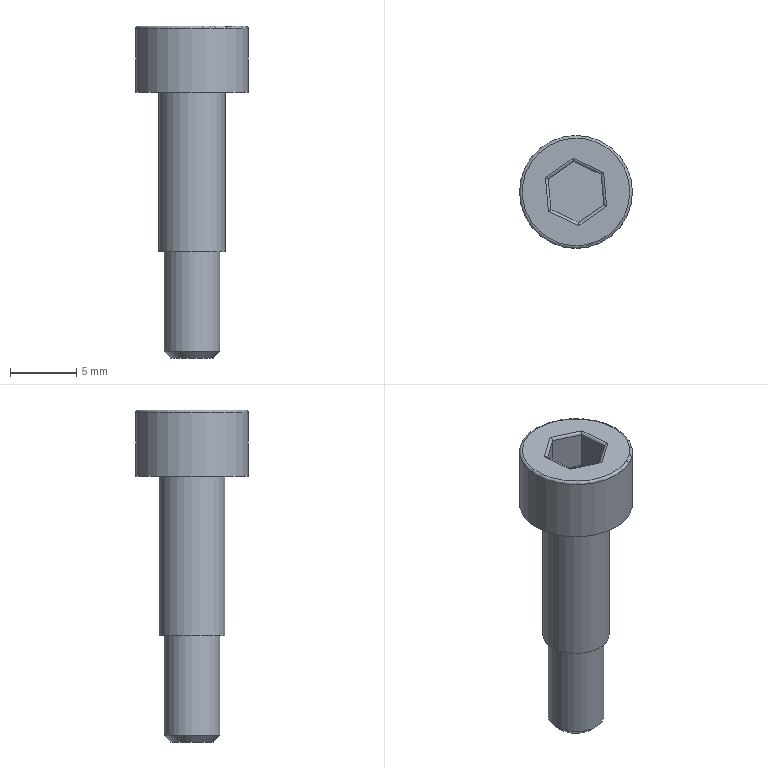Part | STEP file | 200 mesh_id970_x | 1 solid | 22 faces | box 8.5 x 8.5 x 25 mm | volume 586.744 mm3 | plane 11 | cylinder 9 | torus 1 | cone 1 | commonest cylinder face diameters 0.4 x6 4.2 x1 5 x1 8.5 x1
STEP:
#1=CARTESIAN_POINT('',(-16735.184,-4091.769,73.43));
#2=VERTEX_POINT('',#1);
#3=CARTESIAN_POINT('',(-16732.684,-4091.769,73.43));
#4=DIRECTION('',(0.,0.,1.));
#5=DIRECTION('',(-1.,0.,0.));
#6=AXIS2_PLACEMENT_3D('',#3,#4,#5);
#7=CIRCLE('',#6,2.5);
#8=EDGE_CURVE('',#2,#2,#7,.T.);
#9=ORIENTED_EDGE('',*,*,#8,.T.);
#10=EDGE_LOOP('',(#9));
#11=FACE_BOUND('',#10,.T.);
#12=CARTESIAN_POINT('',(-16728.434,-4091.769,73.43));
#13=VERTEX_POINT('',#12);
#14=CARTESIAN_POINT('',(-16732.684,-4091.769,73.43));
#15=DIRECTION('',(0.,0.,1.));
#16=DIRECTION('',(1.,0.,0.));
#17=AXIS2_PLACEMENT_3D('',#14,#15,#16);
#18=CIRCLE('',#17,4.25);
#19=EDGE_CURVE('',#13,#13,#18,.T.);
#20=ORIENTED_EDGE('',*,*,#19,.F.);
#21=EDGE_LOOP('',(#20));
#22=FACE_BOUND('',#21,.T.);
#23=CARTESIAN_POINT('',(-16732.684,-4091.769,73.43));
#24=DIRECTION('',(0.,0.,-1.));
#25=DIRECTION('',(-1.,0.,0.));
#26=AXIS2_PLACEMENT_3D('',#23,#24,#25);
#27=PLANE('',#26);
#28=ADVANCED_FACE('',(#11,#22),#27,.T.);
#29=CARTESIAN_POINT('',(-16734.986,-4090.696,78.43));
#30=VERTEX_POINT('',#29);
#31=CARTESIAN_POINT('',(-16732.905,-4089.239,78.43));
#32=VERTEX_POINT('',#31);
#33=CARTESIAN_POINT('',(-16733.946,-4089.967,78.43));
#34=DIRECTION('',(0.8192,0.5736,0.));
#35=VECTOR('',#34,1.);
#36=LINE('',#33,#35);
#37=EDGE_CURVE('',#30,#32,#36,.T.);
#38=ORIENTED_EDGE('',*,*,#37,.T.);
#39=CARTESIAN_POINT('',(-16730.603,-4090.312,78.43));
#40=VERTEX_POINT('',#39);
#41=CARTESIAN_POINT('',(-16731.754,-4089.775,78.43));
#42=DIRECTION('',(0.9063,-0.4226,0.));
#43=VECTOR('',#42,1.);
#44=LINE('',#41,#43);
#45=EDGE_CURVE('',#32,#40,#44,.T.);
#46=ORIENTED_EDGE('',*,*,#45,.T.);
#47=CARTESIAN_POINT('',(-16730.382,-4092.843,78.43));
#48=VERTEX_POINT('',#47);
#49=CARTESIAN_POINT('',(-16730.492,-4091.577,78.43));
#50=DIRECTION('',(0.08716,-0.9962,0.));
#51=VECTOR('',#50,1.);
#52=LINE('',#49,#51);
#53=EDGE_CURVE('',#40,#48,#52,.T.);
#54=ORIENTED_EDGE('',*,*,#53,.T.);
#55=CARTESIAN_POINT('',(-16732.463,-4094.3,78.43));
#56=VERTEX_POINT('',#55);
#57=CARTESIAN_POINT('',(-16731.422,-4093.571,78.43));
#58=DIRECTION('',(-0.8192,-0.5736,0.));
#59=VECTOR('',#58,1.);
#60=LINE('',#57,#59);
#61=EDGE_CURVE('',#48,#56,#60,.T.);
#62=ORIENTED_EDGE('',*,*,#61,.T.);
#63=CARTESIAN_POINT('',(-16734.765,-4093.226,78.43));
#64=VERTEX_POINT('',#63);
#65=CARTESIAN_POINT('',(-16733.614,-4093.763,78.43));
#66=DIRECTION('',(-0.9063,0.4226,0.));
#67=VECTOR('',#66,1.);
#68=LINE('',#65,#67);
#69=EDGE_CURVE('',#56,#64,#68,.T.);
#70=ORIENTED_EDGE('',*,*,#69,.T.);
#71=CARTESIAN_POINT('',(-16734.876,-4091.961,78.43));
#72=DIRECTION('',(-0.08716,0.9962,0.));
#73=VECTOR('',#72,1.);
#74=LINE('',#71,#73);
#75=EDGE_CURVE('',#64,#30,#74,.T.);
#76=ORIENTED_EDGE('',*,*,#75,.T.);
#77=EDGE_LOOP('',(#38,#46,#54,#62,#70,#76));
#78=FACE_BOUND('',#77,.T.);
#79=CARTESIAN_POINT('',(-16728.634,-4091.769,78.43));
#80=VERTEX_POINT('',#79);
#81=CARTESIAN_POINT('',(-16732.684,-4091.769,78.43));
#82=DIRECTION('',(0.,0.,1.));
#83=DIRECTION('',(1.,0.,0.));
#84=AXIS2_PLACEMENT_3D('',#81,#82,#83);
#85=CIRCLE('',#84,4.05);
#86=EDGE_CURVE('',#80,#80,#85,.T.);
#87=ORIENTED_EDGE('',*,*,#86,.T.);
#88=EDGE_LOOP('',(#87));
#89=FACE_BOUND('',#88,.T.);
#90=CARTESIAN_POINT('',(-16732.684,-4091.769,78.43));
#91=DIRECTION('',(0.,0.,1.));
#92=DIRECTION('',(1.,0.,0.));
#93=AXIS2_PLACEMENT_3D('',#90,#91,#92);
#94=PLANE('',#93);
#95=ADVANCED_FACE('',(#78,#89),#94,.T.);
#96=CARTESIAN_POINT('',(-16728.434,-4091.769,78.23));
#97=VERTEX_POINT('',#96);
#98=CARTESIAN_POINT('',(-16732.684,-4091.769,78.23));
#99=DIRECTION('',(0.,0.,-1.));
#100=DIRECTION('',(1.,0.,0.));
#101=AXIS2_PLACEMENT_3D('',#98,#99,#100);
#102=CIRCLE('',#101,4.25);
#103=EDGE_CURVE('',#97,#97,#102,.T.);
#104=ORIENTED_EDGE('',*,*,#103,.T.);
#105=EDGE_LOOP('',(#104));
#106=FACE_BOUND('',#105,.T.);
#107=ORIENTED_EDGE('',*,*,#19,.T.);
#108=EDGE_LOOP('',(#107));
#109=FACE_BOUND('',#108,.T.);
#110=CARTESIAN_POINT('',(-16732.684,-4091.769,73.43));
#111=DIRECTION('',(0.,0.,1.));
#112=DIRECTION('',(1.,0.,0.));
#113=AXIS2_PLACEMENT_3D('',#110,#111,#112);
#114=CYLINDRICAL_SURFACE('',#113,4.25);
#115=ADVANCED_FACE('',(#106,#109),#114,.T.);
#116=ORIENTED_EDGE('',*,*,#86,.F.);
#117=EDGE_LOOP('',(#116));
#118=FACE_BOUND('',#117,.T.);
#119=ORIENTED_EDGE('',*,*,#103,.F.);
#120=EDGE_LOOP('',(#119));
#121=FACE_BOUND('',#120,.T.);
#122=CARTESIAN_POINT('',(-16732.684,-4091.769,78.23));
#123=DIRECTION('',(0.,0.,1.));
#124=DIRECTION('',(1.,0.,0.));
#125=AXIS2_PLACEMENT_3D('',#122,#123,#124);
#126=TOROIDAL_SURFACE('',#125,4.05,0.2);
#127=ADVANCED_FACE('',(#118,#121),#126,.T.);
#128=CARTESIAN_POINT('',(-16730.591,-4092.745,78.23));
#129=VERTEX_POINT('',#128);
#130=CARTESIAN_POINT('',(-16730.591,-4092.745,75.43));
#131=VERTEX_POINT('',#130);
#132=CARTESIAN_POINT('',(-16730.591,-4092.745,75.43));
#133=DIRECTION('',(0.,0.,-1.));
#134=VECTOR('',#133,1.);
#135=LINE('',#132,#134);
#136=EDGE_CURVE('',#129,#131,#135,.T.);
#137=ORIENTED_EDGE('',*,*,#136,.F.);
#138=CARTESIAN_POINT('',(-16730.792,-4090.445,78.23));
#139=VERTEX_POINT('',#138);
#140=CARTESIAN_POINT('',(-16730.792,-4090.445,78.23));
#141=DIRECTION('',(-0.08716,0.9962,0.));
#142=VECTOR('',#141,1.);
#143=LINE('',#140,#142);
#144=EDGE_CURVE('',#129,#139,#143,.T.);
#145=ORIENTED_EDGE('',*,*,#144,.T.);
#146=CARTESIAN_POINT('',(-16730.792,-4090.445,75.43));
#147=VERTEX_POINT('',#146);
#148=CARTESIAN_POINT('',(-16730.792,-4090.445,75.43));
#149=DIRECTION('',(0.,0.,-1.));
#150=VECTOR('',#149,1.);
#151=LINE('',#148,#150);
#152=EDGE_CURVE('',#139,#147,#151,.T.);
#153=ORIENTED_EDGE('',*,*,#152,.T.);
#154=CARTESIAN_POINT('',(-16730.792,-4090.445,75.43));
#155=DIRECTION('',(-0.08716,0.9962,0.));
#156=VECTOR('',#155,1.);
#157=LINE('',#154,#156);
#158=EDGE_CURVE('',#131,#147,#157,.T.);
#159=ORIENTED_EDGE('',*,*,#158,.F.);
#160=EDGE_LOOP('',(#137,#145,#153,#159));
#161=FACE_OUTER_BOUND('',#160,.T.);
#162=CARTESIAN_POINT('',(-16730.792,-4090.445,75.43));
#163=DIRECTION('',(-0.9962,-0.08716,0.));
#164=DIRECTION('',(0.08716,-0.9962,0.));
#165=AXIS2_PLACEMENT_3D('',#162,#163,#164);
#166=PLANE('',#165);
#167=ADVANCED_FACE('',(#161),#166,.T.);
#168=CARTESIAN_POINT('',(-16732.483,-4094.07,78.23));
#169=VERTEX_POINT('',#168);
#170=CARTESIAN_POINT('',(-16732.483,-4094.07,75.43));
#171=VERTEX_POINT('',#170);
#172=CARTESIAN_POINT('',(-16732.483,-4094.07,75.43));
#173=DIRECTION('',(0.,0.,-1.));
#174=VECTOR('',#173,1.);
#175=LINE('',#172,#174);
#176=EDGE_CURVE('',#169,#171,#175,.T.);
#177=ORIENTED_EDGE('',*,*,#176,.F.);
#178=CARTESIAN_POINT('',(-16730.591,-4092.745,78.23));
#179=DIRECTION('',(0.8192,0.5736,0.));
#180=VECTOR('',#179,1.);
#181=LINE('',#178,#180);
#182=EDGE_CURVE('',#169,#129,#181,.T.);
#183=ORIENTED_EDGE('',*,*,#182,.T.);
#184=ORIENTED_EDGE('',*,*,#136,.T.);
#185=CARTESIAN_POINT('',(-16730.591,-4092.745,75.43));
#186=DIRECTION('',(0.8192,0.5736,0.));
#187=VECTOR('',#186,1.);
#188=LINE('',#185,#187);
#189=EDGE_CURVE('',#171,#131,#188,.T.);
#190=ORIENTED_EDGE('',*,*,#189,.F.);
#191=EDGE_LOOP('',(#177,#183,#184,#190));
#192=FACE_OUTER_BOUND('',#191,.T.);
#193=CARTESIAN_POINT('',(-16730.591,-4092.745,75.43));
#194=DIRECTION('',(-0.5736,0.8192,0.));
#195=DIRECTION('',(-0.8192,-0.5736,0.));
#196=AXIS2_PLACEMENT_3D('',#193,#194,#195);
#197=PLANE('',#196);
#198=ADVANCED_FACE('',(#192),#197,.T.);
#199=CARTESIAN_POINT('',(-16734.576,-4093.094,78.23));
#200=VERTEX_POINT('',#199);
#201=CARTESIAN_POINT('',(-16734.576,-4093.094,75.43));
#202=VERTEX_POINT('',#201);
#203=CARTESIAN_POINT('',(-16734.576,-4093.094,75.43));
#204=DIRECTION('',(0.,0.,-1.));
#205=VECTOR('',#204,1.);
#206=LINE('',#203,#205);
#207=EDGE_CURVE('',#200,#202,#206,.T.);
#208=ORIENTED_EDGE('',*,*,#207,.F.);
#209=CARTESIAN_POINT('',(-16732.483,-4094.07,78.23));
#210=DIRECTION('',(0.9063,-0.4226,0.));
#211=VECTOR('',#210,1.);
#212=LINE('',#209,#211);
#213=EDGE_CURVE('',#200,#169,#212,.T.);
#214=ORIENTED_EDGE('',*,*,#213,.T.);
#215=ORIENTED_EDGE('',*,*,#176,.T.);
#216=CARTESIAN_POINT('',(-16732.483,-4094.07,75.43));
#217=DIRECTION('',(0.9063,-0.4226,0.));
#218=VECTOR('',#217,1.);
#219=LINE('',#216,#218);
#220=EDGE_CURVE('',#202,#171,#219,.T.);
#221=ORIENTED_EDGE('',*,*,#220,.F.);
#222=EDGE_LOOP('',(#208,#214,#215,#221));
#223=FACE_OUTER_BOUND('',#222,.T.);
#224=CARTESIAN_POINT('',(-16732.483,-4094.07,75.43));
#225=DIRECTION('',(0.4226,0.9063,0.));
#226=DIRECTION('',(-0.9063,0.4226,0.));
#227=AXIS2_PLACEMENT_3D('',#224,#225,#226);
#228=PLANE('',#227);
#229=ADVANCED_FACE('',(#223),#228,.T.);
#230=CARTESIAN_POINT('',(-16734.777,-4090.793,78.23));
#231=VERTEX_POINT('',#230);
#232=CARTESIAN_POINT('',(-16734.777,-4090.793,75.43));
#233=VERTEX_POINT('',#232);
#234=CARTESIAN_POINT('',(-16734.777,-4090.793,75.43));
#235=DIRECTION('',(0.,0.,-1.));
#236=VECTOR('',#235,1.);
#237=LINE('',#234,#236);
#238=EDGE_CURVE('',#231,#233,#237,.T.);
#239=ORIENTED_EDGE('',*,*,#238,.F.);
#240=CARTESIAN_POINT('',(-16734.576,-4093.094,78.23));
#241=DIRECTION('',(0.08716,-0.9962,0.));
#242=VECTOR('',#241,1.);
#243=LINE('',#240,#242);
#244=EDGE_CURVE('',#231,#200,#243,.T.);
#245=ORIENTED_EDGE('',*,*,#244,.T.);
#246=ORIENTED_EDGE('',*,*,#207,.T.);
#247=CARTESIAN_POINT('',(-16734.576,-4093.094,75.43));
#248=DIRECTION('',(0.08716,-0.9962,0.));
#249=VECTOR('',#248,1.);
#250=LINE('',#247,#249);
#251=EDGE_CURVE('',#233,#202,#250,.T.);
#252=ORIENTED_EDGE('',*,*,#251,.F.);
#253=EDGE_LOOP('',(#239,#245,#246,#252));
#254=FACE_OUTER_BOUND('',#253,.T.);
#255=CARTESIAN_POINT('',(-16734.576,-4093.094,75.43));
#256=DIRECTION('',(0.9962,0.08716,0.));
#257=DIRECTION('',(-0.08716,0.9962,0.));
#258=AXIS2_PLACEMENT_3D('',#255,#256,#257);
#259=PLANE('',#258);
#260=ADVANCED_FACE('',(#254),#259,.T.);
#261=CARTESIAN_POINT('',(-16732.885,-4089.469,78.23));
#262=VERTEX_POINT('',#261);
#263=CARTESIAN_POINT('',(-16732.885,-4089.469,75.43));
#264=VERTEX_POINT('',#263);
#265=CARTESIAN_POINT('',(-16732.885,-4089.469,75.43));
#266=DIRECTION('',(0.,0.,-1.));
#267=VECTOR('',#266,1.);
#268=LINE('',#265,#267);
#269=EDGE_CURVE('',#262,#264,#268,.T.);
#270=ORIENTED_EDGE('',*,*,#269,.F.);
#271=CARTESIAN_POINT('',(-16734.777,-4090.793,78.23));
#272=DIRECTION('',(-0.8192,-0.5736,0.));
#273=VECTOR('',#272,1.);
#274=LINE('',#271,#273);
#275=EDGE_CURVE('',#262,#231,#274,.T.);
#276=ORIENTED_EDGE('',*,*,#275,.T.);
#277=ORIENTED_EDGE('',*,*,#238,.T.);
#278=CARTESIAN_POINT('',(-16734.777,-4090.793,75.43));
#279=DIRECTION('',(-0.8192,-0.5736,0.));
#280=VECTOR('',#279,1.);
#281=LINE('',#278,#280);
#282=EDGE_CURVE('',#264,#233,#281,.T.);
#283=ORIENTED_EDGE('',*,*,#282,.F.);
#284=EDGE_LOOP('',(#270,#276,#277,#283));
#285=FACE_OUTER_BOUND('',#284,.T.);
#286=CARTESIAN_POINT('',(-16734.777,-4090.793,75.43));
#287=DIRECTION('',(0.5736,-0.8192,0.));
#288=DIRECTION('',(0.8192,0.5736,0.));
#289=AXIS2_PLACEMENT_3D('',#286,#287,#288);
#290=PLANE('',#289);
#291=ADVANCED_FACE('',(#285),#290,.T.);
#292=ORIENTED_EDGE('',*,*,#152,.F.);
#293=CARTESIAN_POINT('',(-16732.885,-4089.469,78.23));
#294=DIRECTION('',(-0.9063,0.4226,0.));
#295=VECTOR('',#294,1.);
#296=LINE('',#293,#295);
#297=EDGE_CURVE('',#139,#262,#296,.T.);
#298=ORIENTED_EDGE('',*,*,#297,.T.);
#299=ORIENTED_EDGE('',*,*,#269,.T.);
#300=CARTESIAN_POINT('',(-16732.885,-4089.469,75.43));
#301=DIRECTION('',(-0.9063,0.4226,0.));
#302=VECTOR('',#301,1.);
#303=LINE('',#300,#302);
#304=EDGE_CURVE('',#147,#264,#303,.T.);
#305=ORIENTED_EDGE('',*,*,#304,.F.);
#306=EDGE_LOOP('',(#292,#298,#299,#305));
#307=FACE_OUTER_BOUND('',#306,.T.);
#308=CARTESIAN_POINT('',(-16732.885,-4089.469,75.43));
#309=DIRECTION('',(-0.4226,-0.9063,0.));
#310=DIRECTION('',(0.9063,-0.4226,0.));
#311=AXIS2_PLACEMENT_3D('',#308,#309,#310);
#312=PLANE('',#311);
#313=ADVANCED_FACE('',(#307),#312,.T.);
#314=ORIENTED_EDGE('',*,*,#158,.T.);
#315=ORIENTED_EDGE('',*,*,#304,.T.);
#316=ORIENTED_EDGE('',*,*,#282,.T.);
#317=ORIENTED_EDGE('',*,*,#251,.T.);
#318=ORIENTED_EDGE('',*,*,#220,.T.);
#319=ORIENTED_EDGE('',*,*,#189,.T.);
#320=EDGE_LOOP('',(#314,#315,#316,#317,#318,#319));
#321=FACE_OUTER_BOUND('',#320,.T.);
#322=CARTESIAN_POINT('',(1.75,-1.5,75.43));
#323=DIRECTION('',(0.,0.,-1.));
#324=DIRECTION('',(-1.,0.,0.));
#325=AXIS2_PLACEMENT_3D('',#322,#323,#324);
#326=PLANE('',#325);
#327=ADVANCED_FACE('',(#321),#326,.F.);
#328=CARTESIAN_POINT('',(-16732.463,-4094.3,78.23));
#329=DIRECTION('',(0.9962,0.08716,0.));
#330=DIRECTION('',(0.08716,-0.9962,0.));
#331=AXIS2_PLACEMENT_3D('',#328,#329,#330);
#332=ELLIPSE('',#331,0.2309,0.2);
#333=EDGE_CURVE('',#169,#56,#332,.T.);
#334=ORIENTED_EDGE('',*,*,#333,.F.);
#335=ORIENTED_EDGE('',*,*,#213,.F.);
#336=CARTESIAN_POINT('',(-16734.765,-4093.226,78.23));
#337=DIRECTION('',(-0.5736,0.8192,0.));
#338=DIRECTION('',(-0.8192,-0.5736,0.));
#339=AXIS2_PLACEMENT_3D('',#336,#337,#338);
#340=ELLIPSE('',#339,0.2309,0.2);
#341=EDGE_CURVE('',#64,#200,#340,.T.);
#342=ORIENTED_EDGE('',*,*,#341,.F.);
#343=ORIENTED_EDGE('',*,*,#69,.F.);
#344=EDGE_LOOP('',(#334,#335,#342,#343));
#345=FACE_OUTER_BOUND('',#344,.T.);
#346=CARTESIAN_POINT('',(-16733.614,-4093.763,78.23));
#347=DIRECTION('',(-0.9063,0.4226,0.));
#348=DIRECTION('',(-0.4226,-0.9063,0.));
#349=AXIS2_PLACEMENT_3D('',#346,#347,#348);
#350=CYLINDRICAL_SURFACE('',#349,0.2);
#351=ADVANCED_FACE('',(#345),#350,.T.);
#352=ORIENTED_EDGE('',*,*,#341,.T.);
#353=ORIENTED_EDGE('',*,*,#244,.F.);
#354=CARTESIAN_POINT('',(-16734.986,-4090.696,78.23));
#355=DIRECTION('',(0.4226,0.9063,0.));
#356=DIRECTION('',(-0.9063,0.4226,0.));
#357=AXIS2_PLACEMENT_3D('',#354,#355,#356);
#358=ELLIPSE('',#357,0.2309,0.2);
#359=EDGE_CURVE('',#30,#231,#358,.T.);
#360=ORIENTED_EDGE('',*,*,#359,.F.);
#361=ORIENTED_EDGE('',*,*,#75,.F.);
#362=EDGE_LOOP('',(#352,#353,#360,#361));
#363=FACE_OUTER_BOUND('',#362,.T.);
#364=CARTESIAN_POINT('',(-16734.876,-4091.961,78.23));
#365=DIRECTION('',(-0.08716,0.9962,0.));
#366=DIRECTION('',(-0.9962,-0.08716,0.));
#367=AXIS2_PLACEMENT_3D('',#364,#365,#366);
#368=CYLINDRICAL_SURFACE('',#367,0.2);
#369=ADVANCED_FACE('',(#363),#368,.T.);
#370=ORIENTED_EDGE('',*,*,#333,.T.);
#371=ORIENTED_EDGE('',*,*,#61,.F.);
#372=CARTESIAN_POINT('',(-16730.382,-4092.843,78.23));
#373=DIRECTION('',(0.4226,0.9063,0.));
#374=DIRECTION('',(0.9063,-0.4226,0.));
#375=AXIS2_PLACEMENT_3D('',#372,#373,#374);
#376=ELLIPSE('',#375,0.2309,0.2);
#377=EDGE_CURVE('',#129,#48,#376,.T.);
#378=ORIENTED_EDGE('',*,*,#377,.F.);
#379=ORIENTED_EDGE('',*,*,#182,.F.);
#380=EDGE_LOOP('',(#370,#371,#378,#379));
#381=FACE_OUTER_BOUND('',#380,.T.);
#382=CARTESIAN_POINT('',(-16731.422,-4093.571,78.23));
#383=DIRECTION('',(-0.8192,-0.5736,0.));
#384=DIRECTION('',(0.5736,-0.8192,0.));
#385=AXIS2_PLACEMENT_3D('',#382,#383,#384);
#386=CYLINDRICAL_SURFACE('',#385,0.2);
#387=ADVANCED_FACE('',(#381),#386,.T.);
#388=ORIENTED_EDGE('',*,*,#359,.T.);
#389=ORIENTED_EDGE('',*,*,#275,.F.);
#390=CARTESIAN_POINT('',(-16732.905,-4089.239,78.23));
#391=DIRECTION('',(0.9962,0.08716,0.));
#392=DIRECTION('',(0.08716,-0.9962,0.));
#393=AXIS2_PLACEMENT_3D('',#390,#391,#392);
#394=ELLIPSE('',#393,0.2309,0.2);
#395=EDGE_CURVE('',#32,#262,#394,.T.);
#396=ORIENTED_EDGE('',*,*,#395,.F.);
#397=ORIENTED_EDGE('',*,*,#37,.F.);
#398=EDGE_LOOP('',(#388,#389,#396,#397));
#399=FACE_OUTER_BOUND('',#398,.T.);
#400=CARTESIAN_POINT('',(-16733.946,-4089.967,78.23));
#401=DIRECTION('',(0.8192,0.5736,0.));
#402=DIRECTION('',(-0.5736,0.8192,0.));
#403=AXIS2_PLACEMENT_3D('',#400,#401,#402);
#404=CYLINDRICAL_SURFACE('',#403,0.2);
#405=ADVANCED_FACE('',(#399),#404,.T.);
#406=ORIENTED_EDGE('',*,*,#377,.T.);
#407=ORIENTED_EDGE('',*,*,#53,.F.);
#408=CARTESIAN_POINT('',(-16730.603,-4090.312,78.23));
#409=DIRECTION('',(-0.5736,0.8192,0.));
#410=DIRECTION('',(0.8192,0.5736,0.));
#411=AXIS2_PLACEMENT_3D('',#408,#409,#410);
#412=ELLIPSE('',#411,0.2309,0.2);
#413=EDGE_CURVE('',#139,#40,#412,.T.);
#414=ORIENTED_EDGE('',*,*,#413,.F.);
#415=ORIENTED_EDGE('',*,*,#144,.F.);
#416=EDGE_LOOP('',(#406,#407,#414,#415));
#417=FACE_OUTER_BOUND('',#416,.T.);
#418=CARTESIAN_POINT('',(-16730.492,-4091.577,78.23));
#419=DIRECTION('',(0.08716,-0.9962,0.));
#420=DIRECTION('',(0.9962,0.08716,0.));
#421=AXIS2_PLACEMENT_3D('',#418,#419,#420);
#422=CYLINDRICAL_SURFACE('',#421,0.2);
#423=ADVANCED_FACE('',(#417),#422,.T.);
#424=ORIENTED_EDGE('',*,*,#395,.T.);
#425=ORIENTED_EDGE('',*,*,#297,.F.);
#426=ORIENTED_EDGE('',*,*,#413,.T.);
#427=ORIENTED_EDGE('',*,*,#45,.F.);
#428=EDGE_LOOP('',(#424,#425,#426,#427));
#429=FACE_OUTER_BOUND('',#428,.T.);
#430=CARTESIAN_POINT('',(-16731.754,-4089.775,78.23));
#431=DIRECTION('',(0.9063,-0.4226,0.));
#432=DIRECTION('',(0.4226,0.9063,0.));
#433=AXIS2_PLACEMENT_3D('',#430,#431,#432);
#434=CYLINDRICAL_SURFACE('',#433,0.2);
#435=ADVANCED_FACE('',(#429),#434,.T.);
#436=CARTESIAN_POINT('',(-16735.184,-4091.769,61.43));
#437=VERTEX_POINT('',#436);
#438=CARTESIAN_POINT('',(-16732.684,-4091.769,61.43));
#439=DIRECTION('',(0.,0.,-1.));
#440=DIRECTION('',(-1.,0.,0.));
#441=AXIS2_PLACEMENT_3D('',#438,#439,#440);
#442=CIRCLE('',#441,2.5);
#443=EDGE_CURVE('',#437,#437,#442,.T.);
#444=ORIENTED_EDGE('',*,*,#443,.F.);
#445=EDGE_LOOP('',(#444));
#446=FACE_BOUND('',#445,.T.);
#447=ORIENTED_EDGE('',*,*,#8,.F.);
#448=EDGE_LOOP('',(#447));
#449=FACE_BOUND('',#448,.T.);
#450=CARTESIAN_POINT('',(-16732.684,-4091.769,73.43));
#451=DIRECTION('',(0.,0.,1.));
#452=DIRECTION('',(1.,0.,0.));
#453=AXIS2_PLACEMENT_3D('',#450,#451,#452);
#454=CYLINDRICAL_SURFACE('',#453,2.5);
#455=ADVANCED_FACE('',(#446,#449),#454,.T.);
#456=ORIENTED_EDGE('',*,*,#443,.T.);
#457=EDGE_LOOP('',(#456));
#458=FACE_BOUND('',#457,.T.);
#459=CARTESIAN_POINT('',(-16734.784,-4091.769,61.43));
#460=VERTEX_POINT('',#459);
#461=CARTESIAN_POINT('',(-16732.684,-4091.769,61.43));
#462=DIRECTION('',(0.,0.,-1.));
#463=DIRECTION('',(-1.,0.,0.));
#464=AXIS2_PLACEMENT_3D('',#461,#462,#463);
#465=CIRCLE('',#464,2.1);
#466=EDGE_CURVE('',#460,#460,#465,.T.);
#467=ORIENTED_EDGE('',*,*,#466,.F.);
#468=EDGE_LOOP('',(#467));
#469=FACE_BOUND('',#468,.T.);
#470=CARTESIAN_POINT('',(-16732.684,-4091.769,61.43));
#471=DIRECTION('',(0.,0.,-1.));
#472=DIRECTION('',(-1.,0.,0.));
#473=AXIS2_PLACEMENT_3D('',#470,#471,#472);
#474=PLANE('',#473);
#475=ADVANCED_FACE('',(#458,#469),#474,.T.);
#476=CARTESIAN_POINT('',(-16734.784,-4091.769,53.93));
#477=VERTEX_POINT('',#476);
#478=CARTESIAN_POINT('',(-16732.684,-4091.769,53.93));
#479=DIRECTION('',(0.,0.,1.));
#480=DIRECTION('',(-1.,0.,0.));
#481=AXIS2_PLACEMENT_3D('',#478,#479,#480);
#482=CIRCLE('',#481,2.1);
#483=EDGE_CURVE('',#477,#477,#482,.T.);
#484=ORIENTED_EDGE('',*,*,#483,.T.);
#485=EDGE_LOOP('',(#484));
#486=FACE_BOUND('',#485,.T.);
#487=ORIENTED_EDGE('',*,*,#466,.T.);
#488=EDGE_LOOP('',(#487));
#489=FACE_BOUND('',#488,.T.);
#490=CARTESIAN_POINT('',(-16732.684,-4091.769,53.43));
#491=DIRECTION('',(0.,0.,1.));
#492=DIRECTION('',(1.,0.,0.));
#493=AXIS2_PLACEMENT_3D('',#490,#491,#492);
#494=CYLINDRICAL_SURFACE('',#493,2.1);
#495=ADVANCED_FACE('',(#486,#489),#494,.T.);
#496=CARTESIAN_POINT('',(-16734.284,-4091.769,53.43));
#497=VERTEX_POINT('',#496);
#498=CARTESIAN_POINT('',(-16732.684,-4091.769,53.43));
#499=DIRECTION('',(0.,0.,-1.));
#500=DIRECTION('',(-1.,0.,0.));
#501=AXIS2_PLACEMENT_3D('',#498,#499,#500);
#502=CIRCLE('',#501,1.6);
#503=EDGE_CURVE('',#497,#497,#502,.T.);
#504=ORIENTED_EDGE('',*,*,#503,.T.);
#505=EDGE_LOOP('',(#504));
#506=FACE_OUTER_BOUND('',#505,.T.);
#507=CARTESIAN_POINT('',(-16732.684,-4091.769,53.43));
#508=DIRECTION('',(0.,0.,-1.));
#509=DIRECTION('',(-1.,0.,0.));
#510=AXIS2_PLACEMENT_3D('',#507,#508,#509);
#511=PLANE('',#510);
#512=ADVANCED_FACE('',(#506),#511,.T.);
#513=ORIENTED_EDGE('',*,*,#503,.F.);
#514=EDGE_LOOP('',(#513));
#515=FACE_BOUND('',#514,.T.);
#516=ORIENTED_EDGE('',*,*,#483,.F.);
#517=EDGE_LOOP('',(#516));
#518=FACE_BOUND('',#517,.T.);
#519=CARTESIAN_POINT('',(-16732.684,-4091.769,53.93));
#520=DIRECTION('',(0.,0.,1.));
#521=DIRECTION('',(1.,0.,0.));
#522=AXIS2_PLACEMENT_3D('',#519,#520,#521);
#523=CONICAL_SURFACE('',#522,2.1,45.);
#524=ADVANCED_FACE('',(#515,#518),#523,.T.);
#525=CLOSED_SHELL('',(#28,#95,#115,#127,#167,#198,#229,#260,#291,#313,#327,#351,#369,#387,#405,#423,#435,#455,#475,#495,#512,#524));
#526=MANIFOLD_SOLID_BREP('',#525);
#527=(LENGTH_UNIT()NAMED_UNIT(*)SI_UNIT(.MILLI.,.METRE.));
#528=UNCERTAINTY_MEASURE_WITH_UNIT(LENGTH_MEASURE(0.00002),#527,'','');
#529=(NAMED_UNIT(*)PLANE_ANGLE_UNIT()SI_UNIT($,.RADIAN.));
#530=PLANE_ANGLE_MEASURE_WITH_UNIT(PLANE_ANGLE_MEASURE(0.01745),#529);
#531=DIMENSIONAL_EXPONENTS(0.,0.,0.,0.,0.,0.,0.);
#532=(CONVERSION_BASED_UNIT('DEGREE',#530)NAMED_UNIT(#531)PLANE_ANGLE_UNIT());
#533=(NAMED_UNIT(*)SI_UNIT($,.STERADIAN.)SOLID_ANGLE_UNIT());
#534=(GEOMETRIC_REPRESENTATION_CONTEXT(3)GLOBAL_UNCERTAINTY_ASSIGNED_CONTEXT((#528))GLOBAL_UNIT_ASSIGNED_CONTEXT((#527,#532,#533))REPRESENTATION_CONTEXT('',''));
#535=ADVANCED_BREP_SHAPE_REPRESENTATION('',(#526),#534);